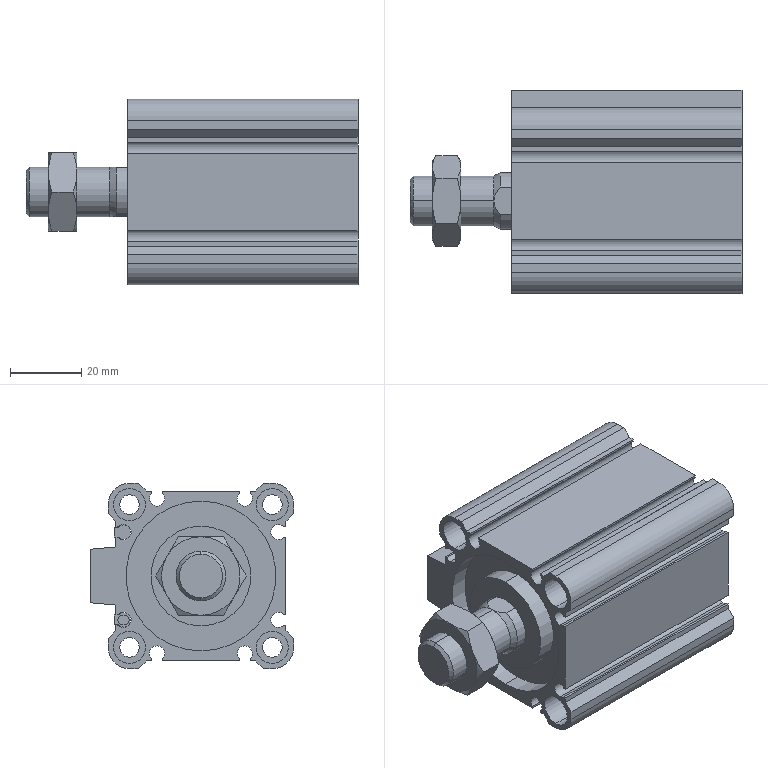Part | SolidWorks | features BaseBody 5 | 5 solids | 236 faces | box 93 x 57 x 52 mm | volume 118892 mm3 | plane 118 | cylinder 94 | cone 24 | commonest cylinder face diameters 4.26 x18 9 x16 0.6 x8 5.5 x8 4 x6 2 x4